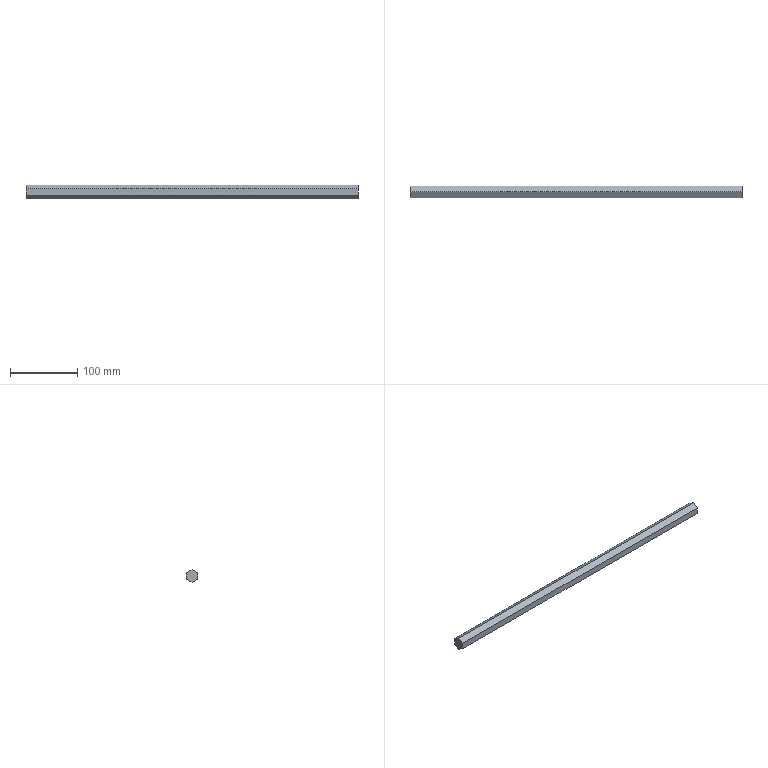Part | STEP file | JBJ-P-1002-05 | 1 solid | 8 faces | box 493 x 17 x 19.63 mm | volume 123389 mm3 | plane 8
STEP:
#1=CARTESIAN_POINT('',(0.,-8.5,4.907));
#2=VERTEX_POINT('',#1);
#3=CARTESIAN_POINT('',(0.,-8.5,-4.907));
#4=VERTEX_POINT('',#3);
#5=CARTESIAN_POINT('',(0.,-8.5,4.907));
#6=DIRECTION('',(0.,0.,-1.));
#7=VECTOR('',#6,1000.);
#8=LINE('',#5,#7);
#9=EDGE_CURVE('',#2,#4,#8,.T.);
#10=ORIENTED_EDGE('',*,*,#9,.T.);
#11=CARTESIAN_POINT('',(493.,-8.5,-4.907));
#12=VERTEX_POINT('',#11);
#13=CARTESIAN_POINT('',(493.,-8.5,-4.907));
#14=DIRECTION('',(-1.,0.,0.));
#15=VECTOR('',#14,1000.);
#16=LINE('',#13,#15);
#17=EDGE_CURVE('',#12,#4,#16,.T.);
#18=ORIENTED_EDGE('',*,*,#17,.F.);
#19=CARTESIAN_POINT('',(493.,-8.5,4.907));
#20=VERTEX_POINT('',#19);
#21=CARTESIAN_POINT('',(493.,-8.5,4.907));
#22=DIRECTION('',(0.,0.,-1.));
#23=VECTOR('',#22,1000.);
#24=LINE('',#21,#23);
#25=EDGE_CURVE('',#20,#12,#24,.T.);
#26=ORIENTED_EDGE('',*,*,#25,.F.);
#27=CARTESIAN_POINT('',(493.,-8.5,4.907));
#28=DIRECTION('',(-1.,0.,0.));
#29=VECTOR('',#28,1000.);
#30=LINE('',#27,#29);
#31=EDGE_CURVE('',#20,#2,#30,.T.);
#32=ORIENTED_EDGE('',*,*,#31,.T.);
#33=EDGE_LOOP('',(#10,#18,#26,#32));
#34=FACE_OUTER_BOUND('',#33,.T.);
#35=CARTESIAN_POINT('',(493.,-8.5,4.907));
#36=DIRECTION('',(0.,1.,0.));
#37=DIRECTION('',(0.,0.,1.));
#38=AXIS2_PLACEMENT_3D('',#35,#36,#37);
#39=PLANE('',#38);
#40=ADVANCED_FACE('',(#34),#39,.F.);
#41=CARTESIAN_POINT('',(0.,0.,-9.815));
#42=VERTEX_POINT('',#41);
#43=CARTESIAN_POINT('',(0.,-8.5,-4.907));
#44=DIRECTION('',(0.,0.866,-0.5));
#45=VECTOR('',#44,1000.);
#46=LINE('',#43,#45);
#47=EDGE_CURVE('',#4,#42,#46,.T.);
#48=ORIENTED_EDGE('',*,*,#47,.T.);
#49=CARTESIAN_POINT('',(493.,0.,-9.815));
#50=VERTEX_POINT('',#49);
#51=CARTESIAN_POINT('',(493.,0.,-9.815));
#52=DIRECTION('',(-1.,0.,0.));
#53=VECTOR('',#52,1000.);
#54=LINE('',#51,#53);
#55=EDGE_CURVE('',#50,#42,#54,.T.);
#56=ORIENTED_EDGE('',*,*,#55,.F.);
#57=CARTESIAN_POINT('',(493.,-8.5,-4.907));
#58=DIRECTION('',(0.,0.866,-0.5));
#59=VECTOR('',#58,1000.);
#60=LINE('',#57,#59);
#61=EDGE_CURVE('',#12,#50,#60,.T.);
#62=ORIENTED_EDGE('',*,*,#61,.F.);
#63=ORIENTED_EDGE('',*,*,#17,.T.);
#64=EDGE_LOOP('',(#48,#56,#62,#63));
#65=FACE_OUTER_BOUND('',#64,.T.);
#66=CARTESIAN_POINT('',(493.,-8.5,-4.907));
#67=DIRECTION('',(0.,0.5,0.866));
#68=DIRECTION('',(0.,-0.866,0.5));
#69=AXIS2_PLACEMENT_3D('',#66,#67,#68);
#70=PLANE('',#69);
#71=ADVANCED_FACE('',(#65),#70,.F.);
#72=CARTESIAN_POINT('',(0.,8.5,-4.907));
#73=VERTEX_POINT('',#72);
#74=CARTESIAN_POINT('',(0.,0.,-9.815));
#75=DIRECTION('',(0.,0.866,0.5));
#76=VECTOR('',#75,1000.);
#77=LINE('',#74,#76);
#78=EDGE_CURVE('',#42,#73,#77,.T.);
#79=ORIENTED_EDGE('',*,*,#78,.T.);
#80=CARTESIAN_POINT('',(493.,8.5,-4.907));
#81=VERTEX_POINT('',#80);
#82=CARTESIAN_POINT('',(493.,8.5,-4.907));
#83=DIRECTION('',(-1.,0.,0.));
#84=VECTOR('',#83,1000.);
#85=LINE('',#82,#84);
#86=EDGE_CURVE('',#81,#73,#85,.T.);
#87=ORIENTED_EDGE('',*,*,#86,.F.);
#88=CARTESIAN_POINT('',(493.,0.,-9.815));
#89=DIRECTION('',(0.,0.866,0.5));
#90=VECTOR('',#89,1000.);
#91=LINE('',#88,#90);
#92=EDGE_CURVE('',#50,#81,#91,.T.);
#93=ORIENTED_EDGE('',*,*,#92,.F.);
#94=ORIENTED_EDGE('',*,*,#55,.T.);
#95=EDGE_LOOP('',(#79,#87,#93,#94));
#96=FACE_OUTER_BOUND('',#95,.T.);
#97=CARTESIAN_POINT('',(493.,0.,-9.815));
#98=DIRECTION('',(0.,-0.5,0.866));
#99=DIRECTION('',(0.,-0.866,-0.5));
#100=AXIS2_PLACEMENT_3D('',#97,#98,#99);
#101=PLANE('',#100);
#102=ADVANCED_FACE('',(#96),#101,.F.);
#103=CARTESIAN_POINT('',(0.,8.5,4.907));
#104=VERTEX_POINT('',#103);
#105=CARTESIAN_POINT('',(0.,8.5,-4.907));
#106=DIRECTION('',(0.,0.,1.));
#107=VECTOR('',#106,1000.);
#108=LINE('',#105,#107);
#109=EDGE_CURVE('',#73,#104,#108,.T.);
#110=ORIENTED_EDGE('',*,*,#109,.T.);
#111=CARTESIAN_POINT('',(493.,8.5,4.907));
#112=VERTEX_POINT('',#111);
#113=CARTESIAN_POINT('',(493.,8.5,4.907));
#114=DIRECTION('',(-1.,0.,0.));
#115=VECTOR('',#114,1000.);
#116=LINE('',#113,#115);
#117=EDGE_CURVE('',#112,#104,#116,.T.);
#118=ORIENTED_EDGE('',*,*,#117,.F.);
#119=CARTESIAN_POINT('',(493.,8.5,-4.907));
#120=DIRECTION('',(0.,0.,1.));
#121=VECTOR('',#120,1000.);
#122=LINE('',#119,#121);
#123=EDGE_CURVE('',#81,#112,#122,.T.);
#124=ORIENTED_EDGE('',*,*,#123,.F.);
#125=ORIENTED_EDGE('',*,*,#86,.T.);
#126=EDGE_LOOP('',(#110,#118,#124,#125));
#127=FACE_OUTER_BOUND('',#126,.T.);
#128=CARTESIAN_POINT('',(493.,8.5,-4.907));
#129=DIRECTION('',(0.,-1.,0.));
#130=DIRECTION('',(0.,0.,-1.));
#131=AXIS2_PLACEMENT_3D('',#128,#129,#130);
#132=PLANE('',#131);
#133=ADVANCED_FACE('',(#127),#132,.F.);
#134=CARTESIAN_POINT('',(0.,0.,9.815));
#135=VERTEX_POINT('',#134);
#136=CARTESIAN_POINT('',(0.,8.5,4.907));
#137=DIRECTION('',(0.,-0.866,0.5));
#138=VECTOR('',#137,1000.);
#139=LINE('',#136,#138);
#140=EDGE_CURVE('',#104,#135,#139,.T.);
#141=ORIENTED_EDGE('',*,*,#140,.T.);
#142=CARTESIAN_POINT('',(493.,0.,9.815));
#143=VERTEX_POINT('',#142);
#144=CARTESIAN_POINT('',(493.,0.,9.815));
#145=DIRECTION('',(-1.,0.,0.));
#146=VECTOR('',#145,1000.);
#147=LINE('',#144,#146);
#148=EDGE_CURVE('',#143,#135,#147,.T.);
#149=ORIENTED_EDGE('',*,*,#148,.F.);
#150=CARTESIAN_POINT('',(493.,8.5,4.907));
#151=DIRECTION('',(0.,-0.866,0.5));
#152=VECTOR('',#151,1000.);
#153=LINE('',#150,#152);
#154=EDGE_CURVE('',#112,#143,#153,.T.);
#155=ORIENTED_EDGE('',*,*,#154,.F.);
#156=ORIENTED_EDGE('',*,*,#117,.T.);
#157=EDGE_LOOP('',(#141,#149,#155,#156));
#158=FACE_OUTER_BOUND('',#157,.T.);
#159=CARTESIAN_POINT('',(493.,8.5,4.907));
#160=DIRECTION('',(0.,-0.5,-0.866));
#161=DIRECTION('',(0.,0.866,-0.5));
#162=AXIS2_PLACEMENT_3D('',#159,#160,#161);
#163=PLANE('',#162);
#164=ADVANCED_FACE('',(#158),#163,.F.);
#165=CARTESIAN_POINT('',(0.,0.,9.815));
#166=DIRECTION('',(0.,-0.866,-0.5));
#167=VECTOR('',#166,1000.);
#168=LINE('',#165,#167);
#169=EDGE_CURVE('',#135,#2,#168,.T.);
#170=ORIENTED_EDGE('',*,*,#169,.T.);
#171=ORIENTED_EDGE('',*,*,#31,.F.);
#172=CARTESIAN_POINT('',(493.,0.,9.815));
#173=DIRECTION('',(0.,-0.866,-0.5));
#174=VECTOR('',#173,1000.);
#175=LINE('',#172,#174);
#176=EDGE_CURVE('',#143,#20,#175,.T.);
#177=ORIENTED_EDGE('',*,*,#176,.F.);
#178=ORIENTED_EDGE('',*,*,#148,.T.);
#179=EDGE_LOOP('',(#170,#171,#177,#178));
#180=FACE_OUTER_BOUND('',#179,.T.);
#181=CARTESIAN_POINT('',(493.,0.,9.815));
#182=DIRECTION('',(0.,0.5,-0.866));
#183=DIRECTION('',(0.,0.866,0.5));
#184=AXIS2_PLACEMENT_3D('',#181,#182,#183);
#185=PLANE('',#184);
#186=ADVANCED_FACE('',(#180),#185,.F.);
#187=ORIENTED_EDGE('',*,*,#25,.T.);
#188=ORIENTED_EDGE('',*,*,#61,.T.);
#189=ORIENTED_EDGE('',*,*,#92,.T.);
#190=ORIENTED_EDGE('',*,*,#123,.T.);
#191=ORIENTED_EDGE('',*,*,#154,.T.);
#192=ORIENTED_EDGE('',*,*,#176,.T.);
#193=EDGE_LOOP('',(#187,#188,#189,#190,#191,#192));
#194=FACE_OUTER_BOUND('',#193,.T.);
#195=CARTESIAN_POINT('',(493.,0.,0.));
#196=DIRECTION('',(1.,0.,0.));
#197=DIRECTION('',(0.,0.,-1.));
#198=AXIS2_PLACEMENT_3D('',#195,#196,#197);
#199=PLANE('',#198);
#200=ADVANCED_FACE('',(#194),#199,.T.);
#201=ORIENTED_EDGE('',*,*,#9,.F.);
#202=ORIENTED_EDGE('',*,*,#169,.F.);
#203=ORIENTED_EDGE('',*,*,#140,.F.);
#204=ORIENTED_EDGE('',*,*,#109,.F.);
#205=ORIENTED_EDGE('',*,*,#78,.F.);
#206=ORIENTED_EDGE('',*,*,#47,.F.);
#207=EDGE_LOOP('',(#201,#202,#203,#204,#205,#206));
#208=FACE_OUTER_BOUND('',#207,.T.);
#209=CARTESIAN_POINT('',(0.,0.,0.));
#210=DIRECTION('',(1.,0.,0.));
#211=DIRECTION('',(0.,0.,-1.));
#212=AXIS2_PLACEMENT_3D('',#209,#210,#211);
#213=PLANE('',#212);
#214=ADVANCED_FACE('',(#208),#213,.F.);
#215=CLOSED_SHELL('',(#40,#71,#102,#133,#164,#186,#200,#214));
#216=MANIFOLD_SOLID_BREP('',#215);
#217=CARTESIAN_POINT('',(0.,0.,0.));
#218=DIRECTION('',(0.,0.,1.));
#219=DIRECTION('',(1.,0.,0.));
#220=AXIS2_PLACEMENT_3D('',#217,#218,#219);
#221=(LENGTH_UNIT()NAMED_UNIT(*)SI_UNIT(.MILLI.,.METRE.));
#222=UNCERTAINTY_MEASURE_WITH_UNIT(LENGTH_MEASURE(0.00001),#221,'','');
#223=(NAMED_UNIT(*)PLANE_ANGLE_UNIT()SI_UNIT($,.RADIAN.));
#224=(NAMED_UNIT(*)SI_UNIT($,.STERADIAN.)SOLID_ANGLE_UNIT());
#225=(GEOMETRIC_REPRESENTATION_CONTEXT(3)GLOBAL_UNCERTAINTY_ASSIGNED_CONTEXT((#222))GLOBAL_UNIT_ASSIGNED_CONTEXT((#221,#223,#224))REPRESENTATION_CONTEXT('',''));
#226=ADVANCED_BREP_SHAPE_REPRESENTATION('',(#216,#220),#225);